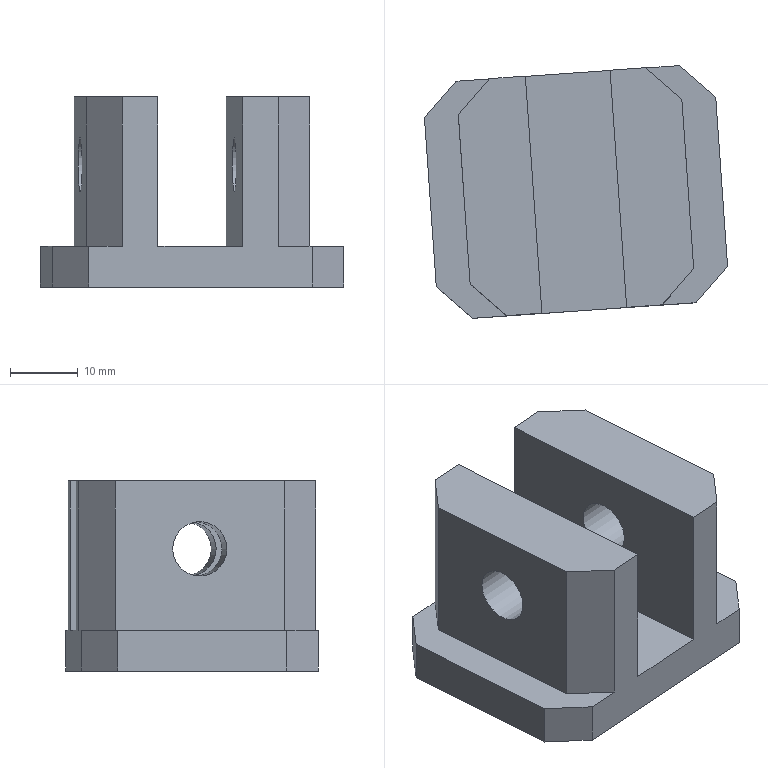Part | STEP file | 车灯-后视镜_id438_x_t | 1 solid | 24 faces | box 44.639 x 37.217 x 28 mm | volume 22385 mm3 | plane 22 | cylinder 2 | commonest cylinder face diameters 8 x2
STEP:
#1=CARTESIAN_POINT('',(7.846,-67.014,-249.5));
#2=VERTEX_POINT('',#1);
#3=CARTESIAN_POINT('',(-4.623,-67.886,-249.5));
#4=VERTEX_POINT('',#3);
#5=CARTESIAN_POINT('',(21.064,-66.089,-249.5));
#6=DIRECTION('',(-0.9976,-0.06976,0.));
#7=VECTOR('',#6,1.);
#8=LINE('',#5,#7);
#9=EDGE_CURVE('',#2,#4,#8,.T.);
#10=ORIENTED_EDGE('',*,*,#9,.T.);
#11=CARTESIAN_POINT('',(-2.182,-102.8,-249.5));
#12=VERTEX_POINT('',#11);
#13=CARTESIAN_POINT('',(-3.788,-79.825,-249.5));
#14=DIRECTION('',(-0.06976,0.9976,0.));
#15=VECTOR('',#14,1.);
#16=LINE('',#13,#15);
#17=EDGE_CURVE('',#12,#4,#16,.T.);
#18=ORIENTED_EDGE('',*,*,#17,.F.);
#19=CARTESIAN_POINT('',(10.288,-101.928,-249.5));
#20=VERTEX_POINT('',#19);
#21=CARTESIAN_POINT('',(23.506,-101.004,-249.5));
#22=DIRECTION('',(0.9976,0.06976,0.));
#23=VECTOR('',#22,1.);
#24=LINE('',#21,#23);
#25=EDGE_CURVE('',#12,#20,#24,.T.);
#26=ORIENTED_EDGE('',*,*,#25,.T.);
#27=CARTESIAN_POINT('',(8.681,-78.953,-249.5));
#28=DIRECTION('',(0.06976,-0.9976,0.));
#29=VECTOR('',#28,1.);
#30=LINE('',#27,#29);
#31=EDGE_CURVE('',#2,#20,#30,.T.);
#32=ORIENTED_EDGE('',*,*,#31,.F.);
#33=EDGE_LOOP('',(#10,#18,#26,#32));
#34=FACE_OUTER_BOUND('',#33,.T.);
#35=CARTESIAN_POINT('',(21.426,-71.27,-249.5));
#36=DIRECTION('',(0.,0.,1.));
#37=DIRECTION('',(0.06976,-0.9976,0.));
#38=AXIS2_PLACEMENT_3D('',#35,#36,#37);
#39=PLANE('',#38);
#40=ADVANCED_FACE('',(#34),#39,.T.);
#41=CARTESIAN_POINT('',(18.071,-66.299,-249.5));
#42=VERTEX_POINT('',#41);
#43=CARTESIAN_POINT('',(13.084,-66.647,-249.5));
#44=VERTEX_POINT('',#43);
#45=CARTESIAN_POINT('',(5.602,-67.171,-249.5));
#46=DIRECTION('',(-0.9976,-0.06976,0.));
#47=VECTOR('',#46,1.);
#48=LINE('',#45,#47);
#49=EDGE_CURVE('',#42,#44,#48,.T.);
#50=ORIENTED_EDGE('',*,*,#49,.T.);
#51=CARTESIAN_POINT('',(18.42,-71.286,-249.5));
#52=VERTEX_POINT('',#51);
#53=CARTESIAN_POINT('',(13.084,-66.647,-249.5));
#54=DIRECTION('',(-0.7547,0.6561,0.));
#55=VECTOR('',#54,1.);
#56=LINE('',#53,#55);
#57=EDGE_CURVE('',#52,#44,#56,.T.);
#58=ORIENTED_EDGE('',*,*,#57,.F.);
#59=CARTESIAN_POINT('',(20.164,-96.226,-249.5));
#60=VERTEX_POINT('',#59);
#61=CARTESIAN_POINT('',(19.232,-82.898,-249.5));
#62=DIRECTION('',(-0.06976,0.9976,0.));
#63=VECTOR('',#62,1.);
#64=LINE('',#61,#63);
#65=EDGE_CURVE('',#60,#52,#64,.T.);
#66=ORIENTED_EDGE('',*,*,#65,.F.);
#67=CARTESIAN_POINT('',(15.525,-101.562,-249.5));
#68=VERTEX_POINT('',#67);
#69=CARTESIAN_POINT('',(20.164,-96.226,-249.5));
#70=DIRECTION('',(0.6561,0.7547,0.));
#71=VECTOR('',#70,1.);
#72=LINE('',#69,#71);
#73=EDGE_CURVE('',#68,#60,#72,.T.);
#74=ORIENTED_EDGE('',*,*,#73,.F.);
#75=CARTESIAN_POINT('',(20.513,-101.213,-249.5));
#76=VERTEX_POINT('',#75);
#77=CARTESIAN_POINT('',(8.043,-102.085,-249.5));
#78=DIRECTION('',(0.9976,0.06976,0.));
#79=VECTOR('',#78,1.);
#80=LINE('',#77,#79);
#81=EDGE_CURVE('',#68,#76,#80,.T.);
#82=ORIENTED_EDGE('',*,*,#81,.T.);
#83=CARTESIAN_POINT('',(25.152,-95.877,-249.5));
#84=VERTEX_POINT('',#83);
#85=CARTESIAN_POINT('',(25.152,-95.877,-249.5));
#86=DIRECTION('',(-0.6561,-0.7547,0.));
#87=VECTOR('',#86,1.);
#88=LINE('',#85,#87);
#89=EDGE_CURVE('',#84,#76,#88,.T.);
#90=ORIENTED_EDGE('',*,*,#89,.F.);
#91=CARTESIAN_POINT('',(23.408,-70.938,-249.5));
#92=VERTEX_POINT('',#91);
#93=CARTESIAN_POINT('',(23.422,-71.13,-249.5));
#94=DIRECTION('',(-0.06976,0.9976,0.));
#95=VECTOR('',#94,1.);
#96=LINE('',#93,#95);
#97=EDGE_CURVE('',#84,#92,#96,.T.);
#98=ORIENTED_EDGE('',*,*,#97,.T.);
#99=CARTESIAN_POINT('',(18.071,-66.299,-249.5));
#100=DIRECTION('',(0.7547,-0.6561,0.));
#101=VECTOR('',#100,1.);
#102=LINE('',#99,#101);
#103=EDGE_CURVE('',#42,#92,#102,.T.);
#104=ORIENTED_EDGE('',*,*,#103,.F.);
#105=EDGE_LOOP('',(#50,#58,#66,#74,#82,#90,#98,#104));
#106=FACE_OUTER_BOUND('',#105,.T.);
#107=CARTESIAN_POINT('',(5.964,-72.351,-249.5));
#108=DIRECTION('',(0.,0.,1.));
#109=DIRECTION('',(0.06976,-0.9976,0.));
#110=AXIS2_PLACEMENT_3D('',#107,#108,#109);
#111=PLANE('',#110);
#112=ADVANCED_FACE('',(#106),#111,.T.);
#113=CARTESIAN_POINT('',(-19.487,-73.937,-249.5));
#114=VERTEX_POINT('',#113);
#115=CARTESIAN_POINT('',(-17.743,-98.876,-249.5));
#116=VERTEX_POINT('',#115);
#117=CARTESIAN_POINT('',(-19.474,-74.13,-249.5));
#118=DIRECTION('',(0.06976,-0.9976,0.));
#119=VECTOR('',#118,1.);
#120=LINE('',#117,#119);
#121=EDGE_CURVE('',#114,#116,#120,.T.);
#122=ORIENTED_EDGE('',*,*,#121,.T.);
#123=CARTESIAN_POINT('',(-12.407,-103.515,-249.5));
#124=VERTEX_POINT('',#123);
#125=CARTESIAN_POINT('',(-12.407,-103.515,-249.5));
#126=DIRECTION('',(-0.7547,0.6561,0.));
#127=VECTOR('',#126,1.);
#128=LINE('',#125,#127);
#129=EDGE_CURVE('',#124,#116,#128,.T.);
#130=ORIENTED_EDGE('',*,*,#129,.F.);
#131=CARTESIAN_POINT('',(-7.419,-103.167,-249.5));
#132=VERTEX_POINT('',#131);
#133=CARTESIAN_POINT('',(34.978,-100.202,-249.5));
#134=DIRECTION('',(0.9976,0.06976,0.));
#135=VECTOR('',#134,1.);
#136=LINE('',#133,#135);
#137=EDGE_CURVE('',#124,#132,#136,.T.);
#138=ORIENTED_EDGE('',*,*,#137,.T.);
#139=CARTESIAN_POINT('',(-12.755,-98.528,-249.5));
#140=VERTEX_POINT('',#139);
#141=CARTESIAN_POINT('',(-7.419,-103.167,-249.5));
#142=DIRECTION('',(0.7547,-0.6561,0.));
#143=VECTOR('',#142,1.);
#144=LINE('',#141,#143);
#145=EDGE_CURVE('',#140,#132,#144,.T.);
#146=ORIENTED_EDGE('',*,*,#145,.F.);
#147=CARTESIAN_POINT('',(-14.499,-73.588,-249.5));
#148=VERTEX_POINT('',#147);
#149=CARTESIAN_POINT('',(-13.687,-85.2,-249.5));
#150=DIRECTION('',(0.06976,-0.9976,0.));
#151=VECTOR('',#150,1.);
#152=LINE('',#149,#151);
#153=EDGE_CURVE('',#148,#140,#152,.T.);
#154=ORIENTED_EDGE('',*,*,#153,.F.);
#155=CARTESIAN_POINT('',(-9.86,-68.252,-249.5));
#156=VERTEX_POINT('',#155);
#157=CARTESIAN_POINT('',(-14.499,-73.588,-249.5));
#158=DIRECTION('',(-0.6561,-0.7547,0.));
#159=VECTOR('',#158,1.);
#160=LINE('',#157,#159);
#161=EDGE_CURVE('',#156,#148,#160,.T.);
#162=ORIENTED_EDGE('',*,*,#161,.F.);
#163=CARTESIAN_POINT('',(-14.848,-68.601,-249.5));
#164=VERTEX_POINT('',#163);
#165=CARTESIAN_POINT('',(32.536,-65.287,-249.5));
#166=DIRECTION('',(-0.9976,-0.06976,0.));
#167=VECTOR('',#166,1.);
#168=LINE('',#165,#167);
#169=EDGE_CURVE('',#156,#164,#168,.T.);
#170=ORIENTED_EDGE('',*,*,#169,.T.);
#171=CARTESIAN_POINT('',(-19.487,-73.937,-249.5));
#172=DIRECTION('',(0.6561,0.7547,0.));
#173=VECTOR('',#172,1.);
#174=LINE('',#171,#173);
#175=EDGE_CURVE('',#114,#164,#174,.T.);
#176=ORIENTED_EDGE('',*,*,#175,.F.);
#177=EDGE_LOOP('',(#122,#130,#138,#146,#154,#162,#170,#176));
#178=FACE_OUTER_BOUND('',#177,.T.);
#179=CARTESIAN_POINT('',(32.898,-70.468,-249.5));
#180=DIRECTION('',(0.,0.,1.));
#181=DIRECTION('',(0.06976,-0.9976,0.));
#182=AXIS2_PLACEMENT_3D('',#179,#180,#181);
#183=PLANE('',#182);
#184=ADVANCED_FACE('',(#178),#183,.T.);
#185=ORIENTED_EDGE('',*,*,#97,.F.);
#186=CARTESIAN_POINT('',(25.152,-95.877,-255.5));
#187=VERTEX_POINT('',#186);
#188=CARTESIAN_POINT('',(25.152,-95.877,-255.5));
#189=DIRECTION('',(0.,0.,1.));
#190=VECTOR('',#189,1.);
#191=LINE('',#188,#190);
#192=EDGE_CURVE('',#187,#84,#191,.T.);
#193=ORIENTED_EDGE('',*,*,#192,.F.);
#194=CARTESIAN_POINT('',(23.408,-70.938,-255.5));
#195=VERTEX_POINT('',#194);
#196=CARTESIAN_POINT('',(24.22,-82.549,-255.5));
#197=DIRECTION('',(0.06976,-0.9976,0.));
#198=VECTOR('',#197,1.);
#199=LINE('',#196,#198);
#200=EDGE_CURVE('',#195,#187,#199,.T.);
#201=ORIENTED_EDGE('',*,*,#200,.F.);
#202=CARTESIAN_POINT('',(23.408,-70.938,-255.5));
#203=DIRECTION('',(0.,0.,-1.));
#204=VECTOR('',#203,1.);
#205=LINE('',#202,#204);
#206=EDGE_CURVE('',#92,#195,#205,.T.);
#207=ORIENTED_EDGE('',*,*,#206,.F.);
#208=EDGE_LOOP('',(#185,#193,#201,#207));
#209=FACE_OUTER_BOUND('',#208,.T.);
#210=CARTESIAN_POINT('',(24.22,-82.549,-255.5));
#211=DIRECTION('',(0.9976,0.06976,0.));
#212=DIRECTION('',(0.,0.,-1.));
#213=AXIS2_PLACEMENT_3D('',#210,#211,#212);
#214=PLANE('',#213);
#215=ADVANCED_FACE('',(#209),#214,.T.);
#216=CARTESIAN_POINT('',(-14.848,-68.601,-255.5));
#217=VERTEX_POINT('',#216);
#218=CARTESIAN_POINT('',(18.071,-66.299,-255.5));
#219=VERTEX_POINT('',#218);
#220=CARTESIAN_POINT('',(-8.863,-68.182,-255.5));
#221=DIRECTION('',(0.9976,0.06976,0.));
#222=VECTOR('',#221,1.);
#223=LINE('',#220,#222);
#224=EDGE_CURVE('',#217,#219,#223,.T.);
#225=ORIENTED_EDGE('',*,*,#224,.F.);
#226=CARTESIAN_POINT('',(-14.848,-68.601,-255.5));
#227=DIRECTION('',(0.,0.,-1.));
#228=VECTOR('',#227,1.);
#229=LINE('',#226,#228);
#230=EDGE_CURVE('',#164,#217,#229,.T.);
#231=ORIENTED_EDGE('',*,*,#230,.F.);
#232=ORIENTED_EDGE('',*,*,#169,.F.);
#233=CARTESIAN_POINT('',(-9.86,-68.252,-227.5));
#234=VERTEX_POINT('',#233);
#235=CARTESIAN_POINT('',(-9.86,-68.252,-255.5));
#236=DIRECTION('',(0.,0.,-1.));
#237=VECTOR('',#236,1.);
#238=LINE('',#235,#237);
#239=EDGE_CURVE('',#234,#156,#238,.T.);
#240=ORIENTED_EDGE('',*,*,#239,.F.);
#241=CARTESIAN_POINT('',(-4.623,-67.886,-227.5));
#242=VERTEX_POINT('',#241);
#243=CARTESIAN_POINT('',(-4.374,-67.868,-227.5));
#244=DIRECTION('',(-0.9976,-0.06976,0.));
#245=VECTOR('',#244,1.);
#246=LINE('',#243,#245);
#247=EDGE_CURVE('',#242,#234,#246,.T.);
#248=ORIENTED_EDGE('',*,*,#247,.F.);
#249=CARTESIAN_POINT('',(-4.623,-67.886,-255.5));
#250=DIRECTION('',(0.,0.,-1.));
#251=VECTOR('',#250,1.);
#252=LINE('',#249,#251);
#253=EDGE_CURVE('',#242,#4,#252,.T.);
#254=ORIENTED_EDGE('',*,*,#253,.T.);
#255=ORIENTED_EDGE('',*,*,#9,.F.);
#256=CARTESIAN_POINT('',(7.846,-67.014,-227.5));
#257=VERTEX_POINT('',#256);
#258=CARTESIAN_POINT('',(7.846,-67.014,-243.));
#259=DIRECTION('',(0.,0.,-1.));
#260=VECTOR('',#259,1.);
#261=LINE('',#258,#260);
#262=EDGE_CURVE('',#257,#2,#261,.T.);
#263=ORIENTED_EDGE('',*,*,#262,.F.);
#264=CARTESIAN_POINT('',(13.084,-66.647,-227.5));
#265=VERTEX_POINT('',#264);
#266=CARTESIAN_POINT('',(-17.342,-68.775,-227.5));
#267=DIRECTION('',(-0.9976,-0.06976,0.));
#268=VECTOR('',#267,1.);
#269=LINE('',#266,#268);
#270=EDGE_CURVE('',#265,#257,#269,.T.);
#271=ORIENTED_EDGE('',*,*,#270,.F.);
#272=CARTESIAN_POINT('',(13.084,-66.647,-255.5));
#273=DIRECTION('',(0.,0.,1.));
#274=VECTOR('',#273,1.);
#275=LINE('',#272,#274);
#276=EDGE_CURVE('',#44,#265,#275,.T.);
#277=ORIENTED_EDGE('',*,*,#276,.F.);
#278=ORIENTED_EDGE('',*,*,#49,.F.);
#279=CARTESIAN_POINT('',(18.071,-66.299,-255.5));
#280=DIRECTION('',(0.,0.,1.));
#281=VECTOR('',#280,1.);
#282=LINE('',#279,#281);
#283=EDGE_CURVE('',#219,#42,#282,.T.);
#284=ORIENTED_EDGE('',*,*,#283,.F.);
#285=EDGE_LOOP('',(#225,#231,#232,#240,#248,#254,#255,#263,#271,#277,#278,#284));
#286=FACE_OUTER_BOUND('',#285,.T.);
#287=CARTESIAN_POINT('',(-8.863,-68.182,-255.5));
#288=DIRECTION('',(-0.06976,0.9976,0.));
#289=DIRECTION('',(0.,0.,1.));
#290=AXIS2_PLACEMENT_3D('',#287,#288,#289);
#291=PLANE('',#290);
#292=ADVANCED_FACE('',(#286),#291,.T.);
#293=CARTESIAN_POINT('',(-17.743,-98.876,-255.5));
#294=VERTEX_POINT('',#293);
#295=CARTESIAN_POINT('',(-19.487,-73.937,-255.5));
#296=VERTEX_POINT('',#295);
#297=CARTESIAN_POINT('',(-18.675,-85.549,-255.5));
#298=DIRECTION('',(-0.06976,0.9976,0.));
#299=VECTOR('',#298,1.);
#300=LINE('',#297,#299);
#301=EDGE_CURVE('',#294,#296,#300,.T.);
#302=ORIENTED_EDGE('',*,*,#301,.F.);
#303=CARTESIAN_POINT('',(-17.743,-98.876,-255.5));
#304=DIRECTION('',(0.,0.,-1.));
#305=VECTOR('',#304,1.);
#306=LINE('',#303,#305);
#307=EDGE_CURVE('',#116,#294,#306,.T.);
#308=ORIENTED_EDGE('',*,*,#307,.F.);
#309=ORIENTED_EDGE('',*,*,#121,.F.);
#310=CARTESIAN_POINT('',(-19.487,-73.937,-255.5));
#311=DIRECTION('',(0.,0.,1.));
#312=VECTOR('',#311,1.);
#313=LINE('',#310,#312);
#314=EDGE_CURVE('',#296,#114,#313,.T.);
#315=ORIENTED_EDGE('',*,*,#314,.F.);
#316=EDGE_LOOP('',(#302,#308,#309,#315));
#317=FACE_OUTER_BOUND('',#316,.T.);
#318=CARTESIAN_POINT('',(-18.675,-85.549,-255.5));
#319=DIRECTION('',(-0.9976,-0.06976,0.));
#320=DIRECTION('',(0.,0.,1.));
#321=AXIS2_PLACEMENT_3D('',#318,#319,#320);
#322=PLANE('',#321);
#323=ADVANCED_FACE('',(#317),#322,.T.);
#324=ORIENTED_EDGE('',*,*,#81,.F.);
#325=CARTESIAN_POINT('',(15.525,-101.562,-227.5));
#326=VERTEX_POINT('',#325);
#327=CARTESIAN_POINT('',(15.525,-101.562,-255.5));
#328=DIRECTION('',(0.,0.,-1.));
#329=VECTOR('',#328,1.);
#330=LINE('',#327,#329);
#331=EDGE_CURVE('',#326,#68,#330,.T.);
#332=ORIENTED_EDGE('',*,*,#331,.F.);
#333=CARTESIAN_POINT('',(10.288,-101.928,-227.5));
#334=VERTEX_POINT('',#333);
#335=CARTESIAN_POINT('',(-14.901,-103.69,-227.5));
#336=DIRECTION('',(0.9976,0.06976,0.));
#337=VECTOR('',#336,1.);
#338=LINE('',#335,#337);
#339=EDGE_CURVE('',#334,#326,#338,.T.);
#340=ORIENTED_EDGE('',*,*,#339,.F.);
#341=CARTESIAN_POINT('',(10.288,-101.928,-243.));
#342=DIRECTION('',(0.,0.,1.));
#343=VECTOR('',#342,1.);
#344=LINE('',#341,#343);
#345=EDGE_CURVE('',#20,#334,#344,.T.);
#346=ORIENTED_EDGE('',*,*,#345,.F.);
#347=ORIENTED_EDGE('',*,*,#25,.F.);
#348=CARTESIAN_POINT('',(-2.182,-102.8,-227.5));
#349=VERTEX_POINT('',#348);
#350=CARTESIAN_POINT('',(-2.182,-102.8,-255.5));
#351=DIRECTION('',(0.,0.,1.));
#352=VECTOR('',#351,1.);
#353=LINE('',#350,#352);
#354=EDGE_CURVE('',#12,#349,#353,.T.);
#355=ORIENTED_EDGE('',*,*,#354,.T.);
#356=CARTESIAN_POINT('',(-7.419,-103.167,-227.5));
#357=VERTEX_POINT('',#356);
#358=CARTESIAN_POINT('',(-1.932,-102.783,-227.5));
#359=DIRECTION('',(0.9976,0.06976,0.));
#360=VECTOR('',#359,1.);
#361=LINE('',#358,#360);
#362=EDGE_CURVE('',#357,#349,#361,.T.);
#363=ORIENTED_EDGE('',*,*,#362,.F.);
#364=CARTESIAN_POINT('',(-7.419,-103.167,-255.5));
#365=DIRECTION('',(0.,0.,1.));
#366=VECTOR('',#365,1.);
#367=LINE('',#364,#366);
#368=EDGE_CURVE('',#132,#357,#367,.T.);
#369=ORIENTED_EDGE('',*,*,#368,.F.);
#370=ORIENTED_EDGE('',*,*,#137,.F.);
#371=CARTESIAN_POINT('',(-12.407,-103.515,-255.5));
#372=VERTEX_POINT('',#371);
#373=CARTESIAN_POINT('',(-12.407,-103.515,-255.5));
#374=DIRECTION('',(0.,0.,1.));
#375=VECTOR('',#374,1.);
#376=LINE('',#373,#375);
#377=EDGE_CURVE('',#372,#124,#376,.T.);
#378=ORIENTED_EDGE('',*,*,#377,.F.);
#379=CARTESIAN_POINT('',(20.513,-101.213,-255.5));
#380=VERTEX_POINT('',#379);
#381=CARTESIAN_POINT('',(-6.421,-103.097,-255.5));
#382=DIRECTION('',(-0.9976,-0.06976,0.));
#383=VECTOR('',#382,1.);
#384=LINE('',#381,#383);
#385=EDGE_CURVE('',#380,#372,#384,.T.);
#386=ORIENTED_EDGE('',*,*,#385,.F.);
#387=CARTESIAN_POINT('',(20.513,-101.213,-255.5));
#388=DIRECTION('',(0.,0.,-1.));
#389=VECTOR('',#388,1.);
#390=LINE('',#387,#389);
#391=EDGE_CURVE('',#76,#380,#390,.T.);
#392=ORIENTED_EDGE('',*,*,#391,.F.);
#393=EDGE_LOOP('',(#324,#332,#340,#346,#347,#355,#363,#369,#370,#378,#386,#392));
#394=FACE_OUTER_BOUND('',#393,.T.);
#395=CARTESIAN_POINT('',(-6.421,-103.097,-255.5));
#396=DIRECTION('',(0.06976,-0.9976,0.));
#397=DIRECTION('',(0.,0.,-1.));
#398=AXIS2_PLACEMENT_3D('',#395,#396,#397);
#399=PLANE('',#398);
#400=ADVANCED_FACE('',(#394),#399,.T.);
#401=ORIENTED_EDGE('',*,*,#200,.T.);
#402=CARTESIAN_POINT('',(25.152,-95.877,-255.5));
#403=DIRECTION('',(0.6561,0.7547,0.));
#404=VECTOR('',#403,1.);
#405=LINE('',#402,#404);
#406=EDGE_CURVE('',#380,#187,#405,.T.);
#407=ORIENTED_EDGE('',*,*,#406,.F.);
#408=ORIENTED_EDGE('',*,*,#385,.T.);
#409=CARTESIAN_POINT('',(-12.407,-103.515,-255.5));
#410=DIRECTION('',(0.7547,-0.6561,0.));
#411=VECTOR('',#410,1.);
#412=LINE('',#409,#411);
#413=EDGE_CURVE('',#294,#372,#412,.T.);
#414=ORIENTED_EDGE('',*,*,#413,.F.);
#415=ORIENTED_EDGE('',*,*,#301,.T.);
#416=CARTESIAN_POINT('',(-19.487,-73.937,-255.5));
#417=DIRECTION('',(-0.6561,-0.7547,0.));
#418=VECTOR('',#417,1.);
#419=LINE('',#416,#418);
#420=EDGE_CURVE('',#217,#296,#419,.T.);
#421=ORIENTED_EDGE('',*,*,#420,.F.);
#422=ORIENTED_EDGE('',*,*,#224,.T.);
#423=CARTESIAN_POINT('',(18.071,-66.299,-255.5));
#424=DIRECTION('',(-0.7547,0.6561,0.));
#425=VECTOR('',#424,1.);
#426=LINE('',#423,#425);
#427=EDGE_CURVE('',#195,#219,#426,.T.);
#428=ORIENTED_EDGE('',*,*,#427,.F.);
#429=EDGE_LOOP('',(#401,#407,#408,#414,#415,#421,#422,#428));
#430=FACE_OUTER_BOUND('',#429,.T.);
#431=CARTESIAN_POINT('',(-7.702,-84.782,-255.5));
#432=DIRECTION('',(0.,0.,-1.));
#433=DIRECTION('',(-0.06976,0.9976,0.));
#434=AXIS2_PLACEMENT_3D('',#431,#432,#433);
#435=PLANE('',#434);
#436=ADVANCED_FACE('',(#430),#435,.T.);
#437=CARTESIAN_POINT('',(-13.348,-90.048,-237.501));
#438=VERTEX_POINT('',#437);
#439=CARTESIAN_POINT('',(-13.627,-86.058,-237.501));
#440=DIRECTION('',(0.9976,0.06976,0.));
#441=DIRECTION('',(0.06976,-0.9976,0.));
#442=AXIS2_PLACEMENT_3D('',#439,#440,#441);
#443=CIRCLE('',#442,4.);
#444=EDGE_CURVE('',#438,#438,#443,.T.);
#445=ORIENTED_EDGE('',*,*,#444,.T.);
#446=EDGE_LOOP('',(#445));
#447=FACE_BOUND('',#446,.T.);
#448=ORIENTED_EDGE('',*,*,#153,.T.);
#449=CARTESIAN_POINT('',(-12.755,-98.528,-227.5));
#450=VERTEX_POINT('',#449);
#451=CARTESIAN_POINT('',(-12.755,-98.528,-255.5));
#452=DIRECTION('',(0.,0.,-1.));
#453=VECTOR('',#452,1.);
#454=LINE('',#451,#453);
#455=EDGE_CURVE('',#450,#140,#454,.T.);
#456=ORIENTED_EDGE('',*,*,#455,.F.);
#457=CARTESIAN_POINT('',(-14.499,-73.588,-227.5));
#458=VERTEX_POINT('',#457);
#459=CARTESIAN_POINT('',(-13.687,-85.2,-227.5));
#460=DIRECTION('',(0.06976,-0.9976,0.));
#461=VECTOR('',#460,1.);
#462=LINE('',#459,#461);
#463=EDGE_CURVE('',#458,#450,#462,.T.);
#464=ORIENTED_EDGE('',*,*,#463,.F.);
#465=CARTESIAN_POINT('',(-14.499,-73.588,-255.5));
#466=DIRECTION('',(0.,0.,1.));
#467=VECTOR('',#466,1.);
#468=LINE('',#465,#467);
#469=EDGE_CURVE('',#148,#458,#468,.T.);
#470=ORIENTED_EDGE('',*,*,#469,.F.);
#471=EDGE_LOOP('',(#448,#456,#464,#470));
#472=FACE_BOUND('',#471,.T.);
#473=CARTESIAN_POINT('',(-13.687,-85.2,-255.5));
#474=DIRECTION('',(-0.9976,-0.06976,0.));
#475=DIRECTION('',(0.,0.,1.));
#476=AXIS2_PLACEMENT_3D('',#473,#474,#475);
#477=PLANE('',#476);
#478=ADVANCED_FACE('',(#447,#472),#477,.T.);
#479=CARTESIAN_POINT('',(-3.123,-89.333,-237.501));
#480=VERTEX_POINT('',#479);
#481=CARTESIAN_POINT('',(-3.402,-85.343,-237.501));
#482=DIRECTION('',(0.9976,0.06976,0.));
#483=DIRECTION('',(0.06976,-0.9976,0.));
#484=AXIS2_PLACEMENT_3D('',#481,#482,#483);
#485=CIRCLE('',#484,4.);
#486=EDGE_CURVE('',#480,#480,#485,.T.);
#487=ORIENTED_EDGE('',*,*,#486,.F.);
#488=EDGE_LOOP('',(#487));
#489=FACE_BOUND('',#488,.T.);
#490=CARTESIAN_POINT('',(-3.462,-84.485,-227.5));
#491=DIRECTION('',(-0.06976,0.9976,0.));
#492=VECTOR('',#491,1.);
#493=LINE('',#490,#492);
#494=EDGE_CURVE('',#349,#242,#493,.T.);
#495=ORIENTED_EDGE('',*,*,#494,.F.);
#496=ORIENTED_EDGE('',*,*,#354,.F.);
#497=ORIENTED_EDGE('',*,*,#17,.T.);
#498=ORIENTED_EDGE('',*,*,#253,.F.);
#499=EDGE_LOOP('',(#495,#496,#497,#498));
#500=FACE_BOUND('',#499,.T.);
#501=CARTESIAN_POINT('',(-3.788,-79.825,-243.));
#502=DIRECTION('',(-0.9976,-0.06976,0.));
#503=DIRECTION('',(0.,0.,1.));
#504=AXIS2_PLACEMENT_3D('',#501,#502,#503);
#505=PLANE('',#504);
#506=ADVANCED_FACE('',(#489,#500),#505,.F.);
#507=ORIENTED_EDGE('',*,*,#463,.T.);
#508=CARTESIAN_POINT('',(-7.419,-103.167,-227.5));
#509=DIRECTION('',(-0.7547,0.6561,0.));
#510=VECTOR('',#509,1.);
#511=LINE('',#508,#510);
#512=EDGE_CURVE('',#357,#450,#511,.T.);
#513=ORIENTED_EDGE('',*,*,#512,.F.);
#514=ORIENTED_EDGE('',*,*,#362,.T.);
#515=ORIENTED_EDGE('',*,*,#494,.T.);
#516=ORIENTED_EDGE('',*,*,#247,.T.);
#517=CARTESIAN_POINT('',(-14.499,-73.588,-227.5));
#518=DIRECTION('',(0.6561,0.7547,0.));
#519=VECTOR('',#518,1.);
#520=LINE('',#517,#519);
#521=EDGE_CURVE('',#458,#234,#520,.T.);
#522=ORIENTED_EDGE('',*,*,#521,.F.);
#523=EDGE_LOOP('',(#507,#513,#514,#515,#516,#522));
#524=FACE_OUTER_BOUND('',#523,.T.);
#525=CARTESIAN_POINT('',(-3.213,-84.468,-227.5));
#526=DIRECTION('',(0.,0.,1.));
#527=DIRECTION('',(0.06976,-0.9976,0.));
#528=AXIS2_PLACEMENT_3D('',#525,#526,#527);
#529=PLANE('',#528);
#530=ADVANCED_FACE('',(#524),#529,.T.);
#531=CARTESIAN_POINT('',(20.164,-96.226,-227.5));
#532=VERTEX_POINT('',#531);
#533=CARTESIAN_POINT('',(18.42,-71.286,-227.5));
#534=VERTEX_POINT('',#533);
#535=CARTESIAN_POINT('',(19.232,-82.898,-227.5));
#536=DIRECTION('',(-0.06976,0.9976,0.));
#537=VECTOR('',#536,1.);
#538=LINE('',#535,#537);
#539=EDGE_CURVE('',#532,#534,#538,.T.);
#540=ORIENTED_EDGE('',*,*,#539,.T.);
#541=CARTESIAN_POINT('',(13.084,-66.647,-227.5));
#542=DIRECTION('',(0.7547,-0.6561,0.));
#543=VECTOR('',#542,1.);
#544=LINE('',#541,#543);
#545=EDGE_CURVE('',#265,#534,#544,.T.);
#546=ORIENTED_EDGE('',*,*,#545,.F.);
#547=ORIENTED_EDGE('',*,*,#270,.T.);
#548=CARTESIAN_POINT('',(8.681,-78.953,-227.5));
#549=DIRECTION('',(-0.06976,0.9976,0.));
#550=VECTOR('',#549,1.);
#551=LINE('',#548,#550);
#552=EDGE_CURVE('',#334,#257,#551,.T.);
#553=ORIENTED_EDGE('',*,*,#552,.F.);
#554=ORIENTED_EDGE('',*,*,#339,.T.);
#555=CARTESIAN_POINT('',(20.164,-96.226,-227.5));
#556=DIRECTION('',(-0.6561,-0.7547,0.));
#557=VECTOR('',#556,1.);
#558=LINE('',#555,#557);
#559=EDGE_CURVE('',#532,#326,#558,.T.);
#560=ORIENTED_EDGE('',*,*,#559,.F.);
#561=EDGE_LOOP('',(#540,#546,#547,#553,#554,#560));
#562=FACE_OUTER_BOUND('',#561,.T.);
#563=CARTESIAN_POINT('',(-16.181,-85.374,-227.5));
#564=DIRECTION('',(0.,0.,1.));
#565=DIRECTION('',(0.06976,-0.9976,0.));
#566=AXIS2_PLACEMENT_3D('',#563,#564,#565);
#567=PLANE('',#566);
#568=ADVANCED_FACE('',(#562),#567,.T.);
#569=CARTESIAN_POINT('',(19.013,-79.766,-237.501));
#570=VERTEX_POINT('',#569);
#571=CARTESIAN_POINT('',(19.292,-83.756,-237.501));
#572=DIRECTION('',(-0.9976,-0.06976,0.));
#573=DIRECTION('',(-0.06976,0.9976,0.));
#574=AXIS2_PLACEMENT_3D('',#571,#572,#573);
#575=CIRCLE('',#574,4.);
#576=EDGE_CURVE('',#570,#570,#575,.T.);
#577=ORIENTED_EDGE('',*,*,#576,.T.);
#578=EDGE_LOOP('',(#577));
#579=FACE_BOUND('',#578,.T.);
#580=ORIENTED_EDGE('',*,*,#65,.T.);
#581=CARTESIAN_POINT('',(18.42,-71.286,-255.5));
#582=DIRECTION('',(0.,0.,-1.));
#583=VECTOR('',#582,1.);
#584=LINE('',#581,#583);
#585=EDGE_CURVE('',#534,#52,#584,.T.);
#586=ORIENTED_EDGE('',*,*,#585,.F.);
#587=ORIENTED_EDGE('',*,*,#539,.F.);
#588=CARTESIAN_POINT('',(20.164,-96.226,-255.5));
#589=DIRECTION('',(0.,0.,1.));
#590=VECTOR('',#589,1.);
#591=LINE('',#588,#590);
#592=EDGE_CURVE('',#60,#532,#591,.T.);
#593=ORIENTED_EDGE('',*,*,#592,.F.);
#594=EDGE_LOOP('',(#580,#586,#587,#593));
#595=FACE_BOUND('',#594,.T.);
#596=CARTESIAN_POINT('',(19.232,-82.898,-255.5));
#597=DIRECTION('',(0.9976,0.06976,0.));
#598=DIRECTION('',(0.,0.,-1.));
#599=AXIS2_PLACEMENT_3D('',#596,#597,#598);
#600=PLANE('',#599);
#601=ADVANCED_FACE('',(#579,#595),#600,.T.);
#602=CARTESIAN_POINT('',(8.788,-80.481,-237.501));
#603=VERTEX_POINT('',#602);
#604=CARTESIAN_POINT('',(9.067,-84.471,-237.501));
#605=DIRECTION('',(-0.9976,-0.06976,0.));
#606=DIRECTION('',(-0.06976,0.9976,0.));
#607=AXIS2_PLACEMENT_3D('',#604,#605,#606);
#608=CIRCLE('',#607,4.);
#609=EDGE_CURVE('',#603,#603,#608,.T.);
#610=ORIENTED_EDGE('',*,*,#609,.F.);
#611=EDGE_LOOP('',(#610));
#612=FACE_BOUND('',#611,.T.);
#613=ORIENTED_EDGE('',*,*,#262,.T.);
#614=ORIENTED_EDGE('',*,*,#31,.T.);
#615=ORIENTED_EDGE('',*,*,#345,.T.);
#616=ORIENTED_EDGE('',*,*,#552,.T.);
#617=EDGE_LOOP('',(#613,#614,#615,#616));
#618=FACE_BOUND('',#617,.T.);
#619=CARTESIAN_POINT('',(8.681,-78.953,-243.));
#620=DIRECTION('',(0.9976,0.06976,0.));
#621=DIRECTION('',(0.,0.,-1.));
#622=AXIS2_PLACEMENT_3D('',#619,#620,#621);
#623=PLANE('',#622);
#624=ADVANCED_FACE('',(#612,#618),#623,.F.);
#625=ORIENTED_EDGE('',*,*,#576,.F.);
#626=EDGE_LOOP('',(#625));
#627=FACE_BOUND('',#626,.T.);
#628=ORIENTED_EDGE('',*,*,#609,.T.);
#629=EDGE_LOOP('',(#628));
#630=FACE_BOUND('',#629,.T.);
#631=CARTESIAN_POINT('',(40.643,-82.263,-237.501));
#632=DIRECTION('',(-0.9976,-0.06976,0.));
#633=DIRECTION('',(0.,0.,1.));
#634=AXIS2_PLACEMENT_3D('',#631,#632,#633);
#635=CYLINDRICAL_SURFACE('',#634,4.);
#636=ADVANCED_FACE('',(#627,#630),#635,.F.);
#637=ORIENTED_EDGE('',*,*,#444,.F.);
#638=EDGE_LOOP('',(#637));
#639=FACE_BOUND('',#638,.T.);
#640=ORIENTED_EDGE('',*,*,#486,.T.);
#641=EDGE_LOOP('',(#640));
#642=FACE_BOUND('',#641,.T.);
#643=CARTESIAN_POINT('',(53.611,-81.356,-237.501));
#644=DIRECTION('',(-0.9976,-0.06976,0.));
#645=DIRECTION('',(0.,0.,1.));
#646=AXIS2_PLACEMENT_3D('',#643,#644,#645);
#647=CYLINDRICAL_SURFACE('',#646,4.);
#648=ADVANCED_FACE('',(#639,#642),#647,.F.);
#649=ORIENTED_EDGE('',*,*,#161,.T.);
#650=ORIENTED_EDGE('',*,*,#469,.T.);
#651=ORIENTED_EDGE('',*,*,#521,.T.);
#652=ORIENTED_EDGE('',*,*,#239,.T.);
#653=EDGE_LOOP('',(#649,#650,#651,#652));
#654=FACE_OUTER_BOUND('',#653,.T.);
#655=CARTESIAN_POINT('',(-14.499,-73.588,-255.5));
#656=DIRECTION('',(0.7547,-0.6561,0.));
#657=DIRECTION('',(-0.6561,-0.7547,0.));
#658=AXIS2_PLACEMENT_3D('',#655,#656,#657);
#659=PLANE('',#658);
#660=ADVANCED_FACE('',(#654),#659,.F.);
#661=ORIENTED_EDGE('',*,*,#145,.T.);
#662=ORIENTED_EDGE('',*,*,#368,.T.);
#663=ORIENTED_EDGE('',*,*,#512,.T.);
#664=ORIENTED_EDGE('',*,*,#455,.T.);
#665=EDGE_LOOP('',(#661,#662,#663,#664));
#666=FACE_OUTER_BOUND('',#665,.T.);
#667=CARTESIAN_POINT('',(-7.419,-103.167,-255.5));
#668=DIRECTION('',(0.6561,0.7547,0.));
#669=DIRECTION('',(0.7547,-0.6561,0.));
#670=AXIS2_PLACEMENT_3D('',#667,#668,#669);
#671=PLANE('',#670);
#672=ADVANCED_FACE('',(#666),#671,.F.);
#673=ORIENTED_EDGE('',*,*,#73,.T.);
#674=ORIENTED_EDGE('',*,*,#592,.T.);
#675=ORIENTED_EDGE('',*,*,#559,.T.);
#676=ORIENTED_EDGE('',*,*,#331,.T.);
#677=EDGE_LOOP('',(#673,#674,#675,#676));
#678=FACE_OUTER_BOUND('',#677,.T.);
#679=CARTESIAN_POINT('',(20.164,-96.226,-255.5));
#680=DIRECTION('',(-0.7547,0.6561,0.));
#681=DIRECTION('',(0.6561,0.7547,0.));
#682=AXIS2_PLACEMENT_3D('',#679,#680,#681);
#683=PLANE('',#682);
#684=ADVANCED_FACE('',(#678),#683,.F.);
#685=ORIENTED_EDGE('',*,*,#57,.T.);
#686=ORIENTED_EDGE('',*,*,#276,.T.);
#687=ORIENTED_EDGE('',*,*,#545,.T.);
#688=ORIENTED_EDGE('',*,*,#585,.T.);
#689=EDGE_LOOP('',(#685,#686,#687,#688));
#690=FACE_OUTER_BOUND('',#689,.T.);
#691=CARTESIAN_POINT('',(13.084,-66.647,-255.5));
#692=DIRECTION('',(-0.6561,-0.7547,0.));
#693=DIRECTION('',(-0.7547,0.6561,0.));
#694=AXIS2_PLACEMENT_3D('',#691,#692,#693);
#695=PLANE('',#694);
#696=ADVANCED_FACE('',(#690),#695,.F.);
#697=ORIENTED_EDGE('',*,*,#427,.T.);
#698=ORIENTED_EDGE('',*,*,#283,.T.);
#699=ORIENTED_EDGE('',*,*,#103,.T.);
#700=ORIENTED_EDGE('',*,*,#206,.T.);
#701=EDGE_LOOP('',(#697,#698,#699,#700));
#702=FACE_OUTER_BOUND('',#701,.T.);
#703=CARTESIAN_POINT('',(18.071,-66.299,-255.5));
#704=DIRECTION('',(-0.6561,-0.7547,0.));
#705=DIRECTION('',(-0.7547,0.6561,0.));
#706=AXIS2_PLACEMENT_3D('',#703,#704,#705);
#707=PLANE('',#706);
#708=ADVANCED_FACE('',(#702),#707,.F.);
#709=ORIENTED_EDGE('',*,*,#406,.T.);
#710=ORIENTED_EDGE('',*,*,#192,.T.);
#711=ORIENTED_EDGE('',*,*,#89,.T.);
#712=ORIENTED_EDGE('',*,*,#391,.T.);
#713=EDGE_LOOP('',(#709,#710,#711,#712));
#714=FACE_OUTER_BOUND('',#713,.T.);
#715=CARTESIAN_POINT('',(25.152,-95.877,-255.5));
#716=DIRECTION('',(-0.7547,0.6561,0.));
#717=DIRECTION('',(0.6561,0.7547,0.));
#718=AXIS2_PLACEMENT_3D('',#715,#716,#717);
#719=PLANE('',#718);
#720=ADVANCED_FACE('',(#714),#719,.F.);
#721=ORIENTED_EDGE('',*,*,#420,.T.);
#722=ORIENTED_EDGE('',*,*,#314,.T.);
#723=ORIENTED_EDGE('',*,*,#175,.T.);
#724=ORIENTED_EDGE('',*,*,#230,.T.);
#725=EDGE_LOOP('',(#721,#722,#723,#724));
#726=FACE_OUTER_BOUND('',#725,.T.);
#727=CARTESIAN_POINT('',(-19.487,-73.937,-255.5));
#728=DIRECTION('',(0.7547,-0.6561,0.));
#729=DIRECTION('',(-0.6561,-0.7547,0.));
#730=AXIS2_PLACEMENT_3D('',#727,#728,#729);
#731=PLANE('',#730);
#732=ADVANCED_FACE('',(#726),#731,.F.);
#733=ORIENTED_EDGE('',*,*,#413,.T.);
#734=ORIENTED_EDGE('',*,*,#377,.T.);
#735=ORIENTED_EDGE('',*,*,#129,.T.);
#736=ORIENTED_EDGE('',*,*,#307,.T.);
#737=EDGE_LOOP('',(#733,#734,#735,#736));
#738=FACE_OUTER_BOUND('',#737,.T.);
#739=CARTESIAN_POINT('',(-12.407,-103.515,-255.5));
#740=DIRECTION('',(0.6561,0.7547,0.));
#741=DIRECTION('',(0.7547,-0.6561,0.));
#742=AXIS2_PLACEMENT_3D('',#739,#740,#741);
#743=PLANE('',#742);
#744=ADVANCED_FACE('',(#738),#743,.F.);
#745=CLOSED_SHELL('',(#40,#112,#184,#215,#292,#323,#400,#436,#478,#506,#530,#568,#601,#624,#636,#648,#660,#672,#684,#696,#708,#720,#732,#744));
#746=MANIFOLD_SOLID_BREP('',#745);
#747=(LENGTH_UNIT()NAMED_UNIT(*)SI_UNIT(.MILLI.,.METRE.));
#748=UNCERTAINTY_MEASURE_WITH_UNIT(LENGTH_MEASURE(0.00002),#747,'','');
#749=(NAMED_UNIT(*)PLANE_ANGLE_UNIT()SI_UNIT($,.RADIAN.));
#750=PLANE_ANGLE_MEASURE_WITH_UNIT(PLANE_ANGLE_MEASURE(0.01745),#749);
#751=DIMENSIONAL_EXPONENTS(0.,0.,0.,0.,0.,0.,0.);
#752=(CONVERSION_BASED_UNIT('DEGREE',#750)NAMED_UNIT(#751)PLANE_ANGLE_UNIT());
#753=(NAMED_UNIT(*)SI_UNIT($,.STERADIAN.)SOLID_ANGLE_UNIT());
#754=(GEOMETRIC_REPRESENTATION_CONTEXT(3)GLOBAL_UNCERTAINTY_ASSIGNED_CONTEXT((#748))GLOBAL_UNIT_ASSIGNED_CONTEXT((#747,#752,#753))REPRESENTATION_CONTEXT('',''));
#755=ADVANCED_BREP_SHAPE_REPRESENTATION('',(#746),#754);